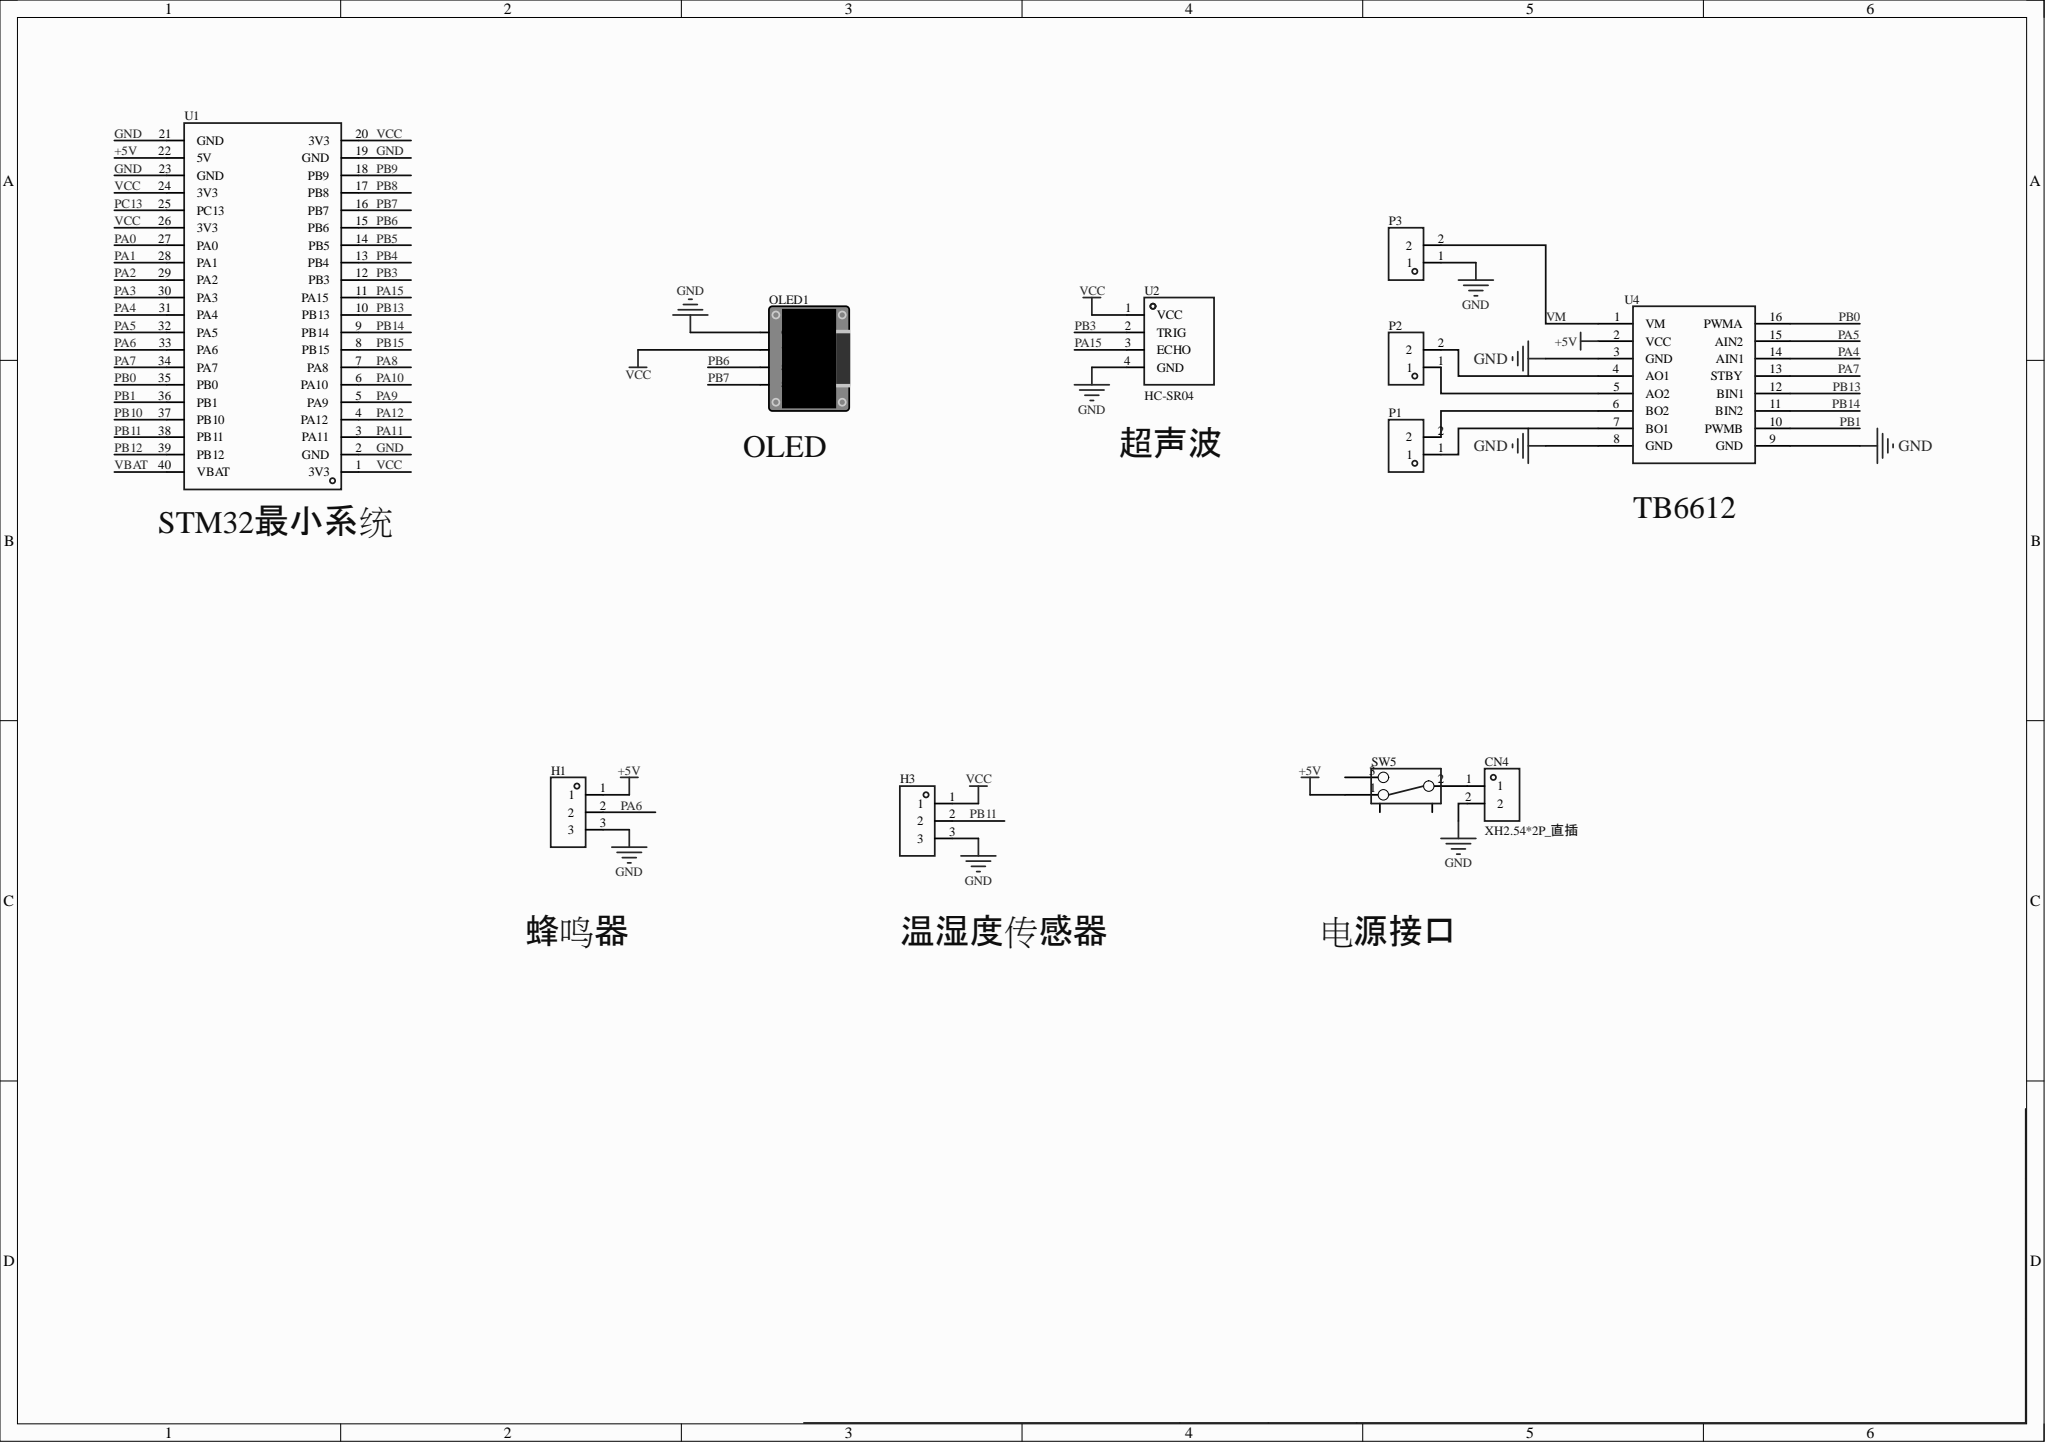Circuit board | Altium Designer | 11 parts | 22 nets
Bill of materials:
Comment,Description,Designator,Footprint,LibRef,Quantity
"XH2.54*2P_直插","","CN4","CONN-TH_2P-P2.50-XH2.54-2P","XH2.54*2P_直插","1"
"","","H1, H3","HDR-TH_3P-P2.54-V-F","HDR-F_2.54_1x3P","2"
"","","OLED1","0.96OLED_4P","0.96OLED模块_4P","1"
"KF301-2P接线端子","","P1, P2, P3","CONN-TH_XY301V-A-5.0-2P","KF301-2P接线端子","3"
"","","SW5","拨动开关","拨动开关_正","1"
"STM32F103C8T6-Card","","U1","CONN-TH_L53.3-W22.9_STM32F103C8T6-CARD","STM32F103C8T6-Card","1"
"HC-SR04","","U2","TH_HC-SR04V","HC-SR04","1"
"","","U4","tb6612","tb6612","1"
Netlist (Protel format):
[
CN4
CONN-TH_2P-P2.50-XH2.54-2P
XH2.54*2P_直插



]
[
H1
HDR-TH_3P-P2.54-V-F




]
[
H3
HDR-TH_3P-P2.54-V-F




]
[
OLED1
0.96OLED_4P




]
[
P1
CONN-TH_XY301V-A-5.0-2P
KF301-2P接线端子



]
[
P2
CONN-TH_XY301V-A-5.0-2P
KF301-2P接线端子



]
[
P3
CONN-TH_XY301V-A-5.0-2P
KF301-2P接线端子



]
[
SW5
拨动开关




]
[
U1
CONN-TH_L53.3-W22.9_STM32F103C8T6-CARD
STM32F103C8T6-Card



]
[
U2
TH_HC-SR04V
HC-SR04



]
[
U4
tb6612




]
(
VM
P3-2
U4-1
)
(
VCC
H3-1
OLED1-2
U1-1
U1-20
U1-24
U1-26
U2-1
)
(
PB14
U1-9
U4-11
)
(
PB13
U1-10
U4-12
)
(
PB11
H3-2
U1-38
)
(
PB7
OLED1-4
U1-16
)
(
PB6
OLED1-3
U1-15
)
(
PB3
U1-12
U2-2
)
(
PB1
U1-36
U4-10
)
(
PB0
U1-35
U4-16
)
(
PA15
U1-11
U2-3
)
(
PA7
U1-34
U4-13
)
(
PA6
H1-2
U1-33
)
(
PA5
U1-32
U4-15
)
(
PA4
U1-31
U4-14
)
(
NetP2_2
P2-2
U4-4
)
(
NetP2_1
P2-1
U4-5
)
(
NetP1_2
P1-2
U4-6
)
(
NetP1_1
P1-1
U4-7
)
(
NetCN4_1
CN4-1
SW5-2
)
(
GND
CN4-2
H1-3
H3-3
OLED1-1
P3-1
U1-2
U1-19
U1-21
U1-23
U2-4
U4-3
U4-8
U4-9
)
(
+5V
H1-1
SW5-1
U1-22
U4-2
)